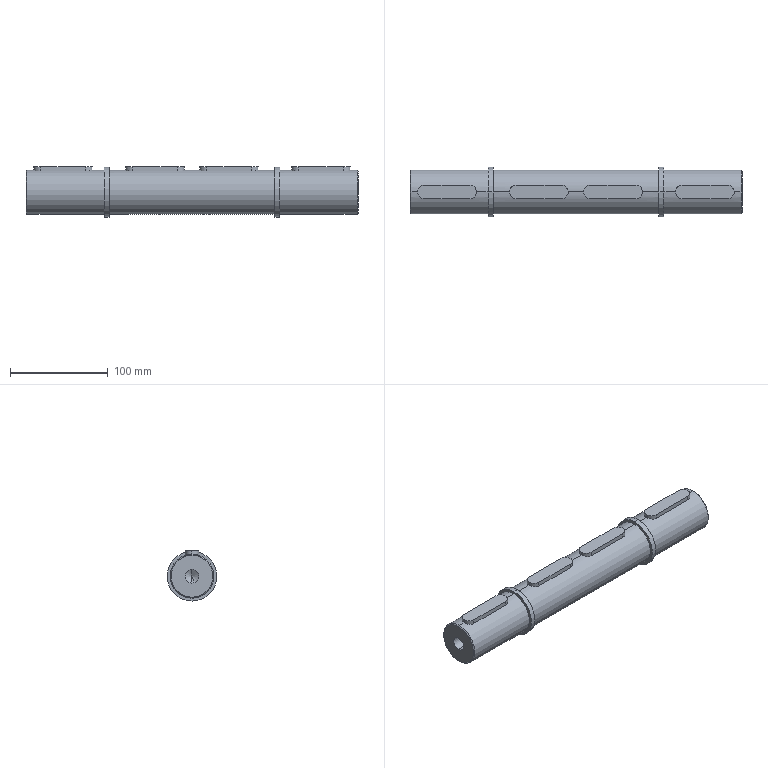Part | SolidWorks | features MirrorPattern 4, Chamfer 1, HoleWzd 1, ICE 1, Revolution 1 | 1 solid | 52 faces | box 340 x 51 x 51.5 mm | volume 551448 mm3 | cylinder 26 | plane 18 | cone 8 | commonest cylinder face diameters 14 x16 45 x6 51 x4